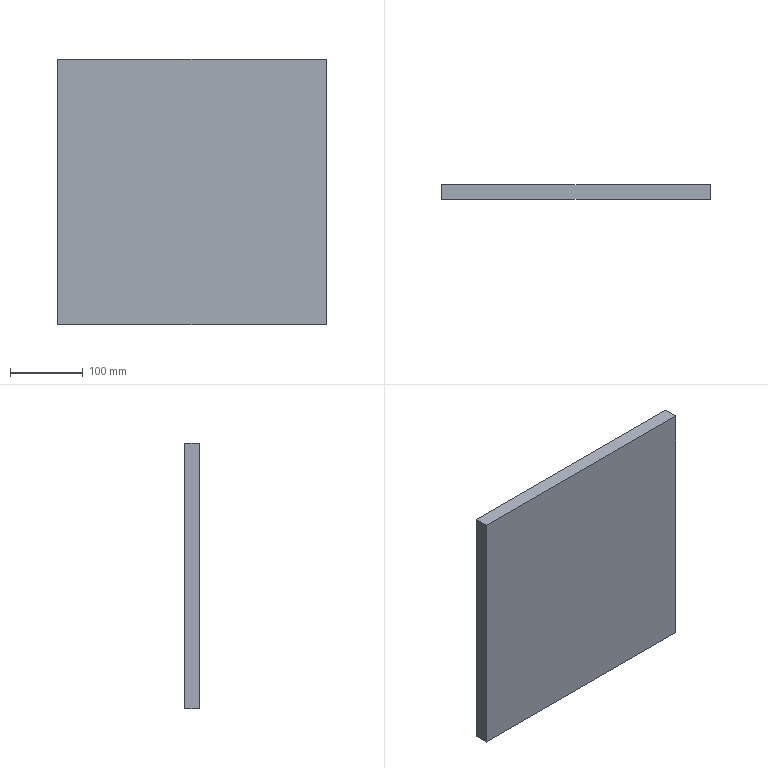Part | SolidWorks | features Extrusion 1 | 1 solid | 6 faces | box 369 x 20 x 365 mm | volume 2693700 mm3 | plane 6
STEP:
#1=CARTESIAN_POINT('',(0.,0.,0.));
#2=VERTEX_POINT('',#1);
#3=CARTESIAN_POINT('',(0.,0.,-365.));
#4=VERTEX_POINT('',#3);
#5=CARTESIAN_POINT('',(0.,0.,0.));
#6=DIRECTION('',(0.,0.,-1.));
#7=VECTOR('',#6,1000.);
#8=LINE('',#5,#7);
#9=EDGE_CURVE('',#2,#4,#8,.T.);
#10=ORIENTED_EDGE('',*,*,#9,.T.);
#11=CARTESIAN_POINT('',(0.,20.,-365.));
#12=VERTEX_POINT('',#11);
#13=CARTESIAN_POINT('',(0.,20.,-365.));
#14=DIRECTION('',(0.,-1.,0.));
#15=VECTOR('',#14,1000.);
#16=LINE('',#13,#15);
#17=EDGE_CURVE('',#12,#4,#16,.T.);
#18=ORIENTED_EDGE('',*,*,#17,.F.);
#19=CARTESIAN_POINT('',(0.,20.,0.));
#20=VERTEX_POINT('',#19);
#21=CARTESIAN_POINT('',(0.,20.,0.));
#22=DIRECTION('',(0.,0.,-1.));
#23=VECTOR('',#22,1000.);
#24=LINE('',#21,#23);
#25=EDGE_CURVE('',#20,#12,#24,.T.);
#26=ORIENTED_EDGE('',*,*,#25,.F.);
#27=CARTESIAN_POINT('',(0.,20.,0.));
#28=DIRECTION('',(0.,-1.,0.));
#29=VECTOR('',#28,1000.);
#30=LINE('',#27,#29);
#31=EDGE_CURVE('',#20,#2,#30,.T.);
#32=ORIENTED_EDGE('',*,*,#31,.T.);
#33=EDGE_LOOP('',(#10,#18,#26,#32));
#34=FACE_OUTER_BOUND('',#33,.T.);
#35=CARTESIAN_POINT('',(0.,20.,0.));
#36=DIRECTION('',(-1.,0.,0.));
#37=DIRECTION('',(0.,0.,1.));
#38=AXIS2_PLACEMENT_3D('',#35,#36,#37);
#39=PLANE('',#38);
#40=ADVANCED_FACE('',(#34),#39,.F.);
#41=CARTESIAN_POINT('',(-369.,0.,-365.));
#42=VERTEX_POINT('',#41);
#43=CARTESIAN_POINT('',(0.,0.,-365.));
#44=DIRECTION('',(-1.,0.,0.));
#45=VECTOR('',#44,1000.);
#46=LINE('',#43,#45);
#47=EDGE_CURVE('',#4,#42,#46,.T.);
#48=ORIENTED_EDGE('',*,*,#47,.T.);
#49=CARTESIAN_POINT('',(-369.,20.,-365.));
#50=VERTEX_POINT('',#49);
#51=CARTESIAN_POINT('',(-369.,20.,-365.));
#52=DIRECTION('',(0.,-1.,0.));
#53=VECTOR('',#52,1000.);
#54=LINE('',#51,#53);
#55=EDGE_CURVE('',#50,#42,#54,.T.);
#56=ORIENTED_EDGE('',*,*,#55,.F.);
#57=CARTESIAN_POINT('',(0.,20.,-365.));
#58=DIRECTION('',(-1.,0.,0.));
#59=VECTOR('',#58,1000.);
#60=LINE('',#57,#59);
#61=EDGE_CURVE('',#12,#50,#60,.T.);
#62=ORIENTED_EDGE('',*,*,#61,.F.);
#63=ORIENTED_EDGE('',*,*,#17,.T.);
#64=EDGE_LOOP('',(#48,#56,#62,#63));
#65=FACE_OUTER_BOUND('',#64,.T.);
#66=CARTESIAN_POINT('',(0.,20.,-365.));
#67=DIRECTION('',(0.,0.,1.));
#68=DIRECTION('',(1.,0.,0.));
#69=AXIS2_PLACEMENT_3D('',#66,#67,#68);
#70=PLANE('',#69);
#71=ADVANCED_FACE('',(#65),#70,.F.);
#72=CARTESIAN_POINT('',(-369.,0.,0.));
#73=VERTEX_POINT('',#72);
#74=CARTESIAN_POINT('',(-369.,0.,0.));
#75=DIRECTION('',(0.,0.,1.));
#76=VECTOR('',#75,1000.);
#77=LINE('',#74,#76);
#78=EDGE_CURVE('',#42,#73,#77,.T.);
#79=ORIENTED_EDGE('',*,*,#78,.T.);
#80=CARTESIAN_POINT('',(-369.,20.,0.));
#81=VERTEX_POINT('',#80);
#82=CARTESIAN_POINT('',(-369.,20.,0.));
#83=DIRECTION('',(0.,-1.,0.));
#84=VECTOR('',#83,1000.);
#85=LINE('',#82,#84);
#86=EDGE_CURVE('',#81,#73,#85,.T.);
#87=ORIENTED_EDGE('',*,*,#86,.F.);
#88=CARTESIAN_POINT('',(-369.,20.,0.));
#89=DIRECTION('',(0.,0.,1.));
#90=VECTOR('',#89,1000.);
#91=LINE('',#88,#90);
#92=EDGE_CURVE('',#50,#81,#91,.T.);
#93=ORIENTED_EDGE('',*,*,#92,.F.);
#94=ORIENTED_EDGE('',*,*,#55,.T.);
#95=EDGE_LOOP('',(#79,#87,#93,#94));
#96=FACE_OUTER_BOUND('',#95,.T.);
#97=CARTESIAN_POINT('',(-369.,20.,0.));
#98=DIRECTION('',(1.,0.,0.));
#99=DIRECTION('',(0.,0.,-1.));
#100=AXIS2_PLACEMENT_3D('',#97,#98,#99);
#101=PLANE('',#100);
#102=ADVANCED_FACE('',(#96),#101,.F.);
#103=CARTESIAN_POINT('',(0.,0.,0.));
#104=DIRECTION('',(1.,0.,0.));
#105=VECTOR('',#104,1000.);
#106=LINE('',#103,#105);
#107=EDGE_CURVE('',#73,#2,#106,.T.);
#108=ORIENTED_EDGE('',*,*,#107,.T.);
#109=ORIENTED_EDGE('',*,*,#31,.F.);
#110=CARTESIAN_POINT('',(0.,20.,0.));
#111=DIRECTION('',(1.,0.,0.));
#112=VECTOR('',#111,1000.);
#113=LINE('',#110,#112);
#114=EDGE_CURVE('',#81,#20,#113,.T.);
#115=ORIENTED_EDGE('',*,*,#114,.F.);
#116=ORIENTED_EDGE('',*,*,#86,.T.);
#117=EDGE_LOOP('',(#108,#109,#115,#116));
#118=FACE_OUTER_BOUND('',#117,.T.);
#119=CARTESIAN_POINT('',(0.,20.,0.));
#120=DIRECTION('',(0.,0.,-1.));
#121=DIRECTION('',(-1.,0.,0.));
#122=AXIS2_PLACEMENT_3D('',#119,#120,#121);
#123=PLANE('',#122);
#124=ADVANCED_FACE('',(#118),#123,.F.);
#125=ORIENTED_EDGE('',*,*,#25,.T.);
#126=ORIENTED_EDGE('',*,*,#61,.T.);
#127=ORIENTED_EDGE('',*,*,#92,.T.);
#128=ORIENTED_EDGE('',*,*,#114,.T.);
#129=EDGE_LOOP('',(#125,#126,#127,#128));
#130=FACE_OUTER_BOUND('',#129,.T.);
#131=CARTESIAN_POINT('',(0.,20.,0.));
#132=DIRECTION('',(0.,1.,0.));
#133=DIRECTION('',(0.,0.,1.));
#134=AXIS2_PLACEMENT_3D('',#131,#132,#133);
#135=PLANE('',#134);
#136=ADVANCED_FACE('',(#130),#135,.T.);
#137=ORIENTED_EDGE('',*,*,#9,.F.);
#138=ORIENTED_EDGE('',*,*,#107,.F.);
#139=ORIENTED_EDGE('',*,*,#78,.F.);
#140=ORIENTED_EDGE('',*,*,#47,.F.);
#141=EDGE_LOOP('',(#137,#138,#139,#140));
#142=FACE_OUTER_BOUND('',#141,.T.);
#143=CARTESIAN_POINT('',(0.,0.,0.));
#144=DIRECTION('',(0.,1.,0.));
#145=DIRECTION('',(0.,0.,1.));
#146=AXIS2_PLACEMENT_3D('',#143,#144,#145);
#147=PLANE('',#146);
#148=ADVANCED_FACE('',(#142),#147,.F.);
#149=CLOSED_SHELL('',(#40,#71,#102,#124,#136,#148));
#150=MANIFOLD_SOLID_BREP('',#149);
#151=CARTESIAN_POINT('',(0.,0.,0.));
#152=DIRECTION('',(0.,0.,1.));
#153=DIRECTION('',(1.,0.,0.));
#154=AXIS2_PLACEMENT_3D('',#151,#152,#153);
#155=(LENGTH_UNIT()NAMED_UNIT(*)SI_UNIT(.MILLI.,.METRE.));
#156=UNCERTAINTY_MEASURE_WITH_UNIT(LENGTH_MEASURE(0.00001),#155,'','');
#157=(NAMED_UNIT(*)PLANE_ANGLE_UNIT()SI_UNIT($,.RADIAN.));
#158=(NAMED_UNIT(*)SI_UNIT($,.STERADIAN.)SOLID_ANGLE_UNIT());
#159=(GEOMETRIC_REPRESENTATION_CONTEXT(3)GLOBAL_UNCERTAINTY_ASSIGNED_CONTEXT((#156))GLOBAL_UNIT_ASSIGNED_CONTEXT((#155,#157,#158))REPRESENTATION_CONTEXT('',''));
#160=ADVANCED_BREP_SHAPE_REPRESENTATION('',(#150,#154),#159);